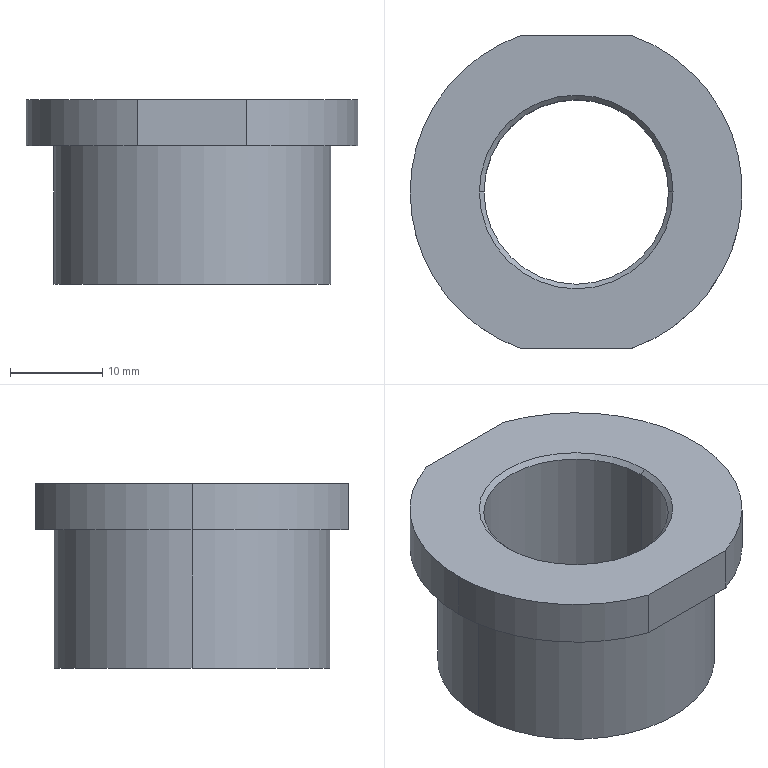Part | SolidWorks | features Chamfer 1, Extrusion 1, ICE 1 | 1 solid | 16 faces | box 36 x 34 x 20 mm | volume 9314 mm3 | cylinder 7 | plane 5 | cone 4 | commonest cylinder face diameters 36 x3 20 x2 30 x2
STEP:
#1=CARTESIAN_POINT('',(-10.,0.,19.5));
#2=VERTEX_POINT('',#1);
#3=CARTESIAN_POINT('',(10.,0.,19.5));
#4=VERTEX_POINT('',#3);
#5=CARTESIAN_POINT('',(0.,0.,19.5));
#6=DIRECTION('',(0.,0.,1.));
#7=DIRECTION('',(1.,0.,0.));
#8=AXIS2_PLACEMENT_3D('',#5,#6,#7);
#9=CIRCLE('',#8,10.);
#10=EDGE_CURVE('',#2,#4,#9,.T.);
#11=ORIENTED_EDGE('',*,*,#10,.F.);
#12=CARTESIAN_POINT('',(-10.5,0.,20.));
#13=VERTEX_POINT('',#12);
#14=CARTESIAN_POINT('',(-10.,0.,19.5));
#15=DIRECTION('',(-0.7071,0.,0.7071));
#16=VECTOR('',#15,1000.);
#17=LINE('',#14,#16);
#18=EDGE_CURVE('',#2,#13,#17,.T.);
#19=ORIENTED_EDGE('',*,*,#18,.T.);
#20=CARTESIAN_POINT('',(10.5,0.,20.));
#21=VERTEX_POINT('',#20);
#22=CARTESIAN_POINT('',(0.,0.,20.));
#23=DIRECTION('',(0.,0.,-1.));
#24=DIRECTION('',(1.,0.,0.));
#25=AXIS2_PLACEMENT_3D('',#22,#23,#24);
#26=CIRCLE('',#25,10.5);
#27=EDGE_CURVE('',#21,#13,#26,.T.);
#28=ORIENTED_EDGE('',*,*,#27,.F.);
#29=CARTESIAN_POINT('',(10.,0.,19.5));
#30=DIRECTION('',(0.7071,0.,0.7071));
#31=VECTOR('',#30,1000.);
#32=LINE('',#29,#31);
#33=EDGE_CURVE('',#4,#21,#32,.T.);
#34=ORIENTED_EDGE('',*,*,#33,.F.);
#35=EDGE_LOOP('',(#11,#19,#28,#34));
#36=FACE_OUTER_BOUND('',#35,.T.);
#37=CARTESIAN_POINT('',(0.,0.,19.5));
#38=DIRECTION('',(0.,0.,1.));
#39=DIRECTION('',(1.,0.,0.));
#40=AXIS2_PLACEMENT_3D('',#37,#38,#39);
#41=CONICAL_SURFACE('',#40,10.,0.7854);
#42=ADVANCED_FACE('',(#36),#41,.F.);
#43=CARTESIAN_POINT('',(10.,0.,0.5));
#44=VERTEX_POINT('',#43);
#45=CARTESIAN_POINT('',(-10.,0.,0.5));
#46=VERTEX_POINT('',#45);
#47=CARTESIAN_POINT('',(0.,0.,0.5));
#48=DIRECTION('',(0.,0.,-1.));
#49=DIRECTION('',(1.,0.,0.));
#50=AXIS2_PLACEMENT_3D('',#47,#48,#49);
#51=CIRCLE('',#50,10.);
#52=EDGE_CURVE('',#44,#46,#51,.T.);
#53=ORIENTED_EDGE('',*,*,#52,.F.);
#54=CARTESIAN_POINT('',(10.5,0.,0.));
#55=VERTEX_POINT('',#54);
#56=CARTESIAN_POINT('',(10.5,0.,0.));
#57=DIRECTION('',(0.7071,0.,-0.7071));
#58=VECTOR('',#57,1000.);
#59=LINE('',#56,#58);
#60=EDGE_CURVE('',#44,#55,#59,.T.);
#61=ORIENTED_EDGE('',*,*,#60,.T.);
#62=CARTESIAN_POINT('',(-10.5,0.,0.));
#63=VERTEX_POINT('',#62);
#64=CARTESIAN_POINT('',(0.,0.,0.));
#65=DIRECTION('',(0.,0.,1.));
#66=DIRECTION('',(1.,0.,0.));
#67=AXIS2_PLACEMENT_3D('',#64,#65,#66);
#68=CIRCLE('',#67,10.5);
#69=EDGE_CURVE('',#63,#55,#68,.T.);
#70=ORIENTED_EDGE('',*,*,#69,.F.);
#71=CARTESIAN_POINT('',(-10.5,0.,0.));
#72=DIRECTION('',(-0.7071,0.,-0.7071));
#73=VECTOR('',#72,1000.);
#74=LINE('',#71,#73);
#75=EDGE_CURVE('',#46,#63,#74,.T.);
#76=ORIENTED_EDGE('',*,*,#75,.F.);
#77=EDGE_LOOP('',(#53,#61,#70,#76));
#78=FACE_OUTER_BOUND('',#77,.T.);
#79=CARTESIAN_POINT('',(0.,0.,0.));
#80=DIRECTION('',(0.,0.,-1.));
#81=DIRECTION('',(-1.,0.,0.));
#82=AXIS2_PLACEMENT_3D('',#79,#80,#81);
#83=CONICAL_SURFACE('',#82,10.5,0.7854);
#84=ADVANCED_FACE('',(#78),#83,.F.);
#85=CARTESIAN_POINT('',(-18.,0.,20.));
#86=VERTEX_POINT('',#85);
#87=CARTESIAN_POINT('',(-5.916,-17.,20.));
#88=VERTEX_POINT('',#87);
#89=CARTESIAN_POINT('',(0.,0.,20.));
#90=DIRECTION('',(0.,0.,1.));
#91=DIRECTION('',(1.,0.,0.));
#92=AXIS2_PLACEMENT_3D('',#89,#90,#91);
#93=CIRCLE('',#92,18.);
#94=EDGE_CURVE('',#86,#88,#93,.T.);
#95=ORIENTED_EDGE('',*,*,#94,.F.);
#96=CARTESIAN_POINT('',(-18.,0.,15.));
#97=VERTEX_POINT('',#96);
#98=CARTESIAN_POINT('',(-18.,0.,20.));
#99=DIRECTION('',(0.,0.,-1.));
#100=VECTOR('',#99,1000.);
#101=LINE('',#98,#100);
#102=EDGE_CURVE('',#86,#97,#101,.T.);
#103=ORIENTED_EDGE('',*,*,#102,.T.);
#104=CARTESIAN_POINT('',(-5.916,-17.,15.));
#105=VERTEX_POINT('',#104);
#106=CARTESIAN_POINT('',(0.,0.,15.));
#107=DIRECTION('',(0.,0.,1.));
#108=DIRECTION('',(1.,0.,0.));
#109=AXIS2_PLACEMENT_3D('',#106,#107,#108);
#110=CIRCLE('',#109,18.);
#111=EDGE_CURVE('',#97,#105,#110,.T.);
#112=ORIENTED_EDGE('',*,*,#111,.T.);
#113=CARTESIAN_POINT('',(-5.916,-17.,20.));
#114=DIRECTION('',(0.,0.,-1.));
#115=VECTOR('',#114,1000.);
#116=LINE('',#113,#115);
#117=EDGE_CURVE('',#88,#105,#116,.T.);
#118=ORIENTED_EDGE('',*,*,#117,.F.);
#119=EDGE_LOOP('',(#95,#103,#112,#118));
#120=FACE_OUTER_BOUND('',#119,.T.);
#121=CARTESIAN_POINT('',(0.,0.,20.));
#122=DIRECTION('',(0.,0.,-1.));
#123=DIRECTION('',(-1.,0.,0.));
#124=AXIS2_PLACEMENT_3D('',#121,#122,#123);
#125=CYLINDRICAL_SURFACE('',#124,18.);
#126=ADVANCED_FACE('',(#120),#125,.T.);
#127=ORIENTED_EDGE('',*,*,#10,.T.);
#128=CARTESIAN_POINT('',(10.,0.,15.));
#129=DIRECTION('',(0.,0.,-1.));
#130=VECTOR('',#129,1000.);
#131=LINE('',#128,#130);
#132=EDGE_CURVE('',#4,#44,#131,.T.);
#133=ORIENTED_EDGE('',*,*,#132,.T.);
#134=ORIENTED_EDGE('',*,*,#52,.T.);
#135=CARTESIAN_POINT('',(-10.,0.,15.));
#136=DIRECTION('',(0.,0.,-1.));
#137=VECTOR('',#136,1000.);
#138=LINE('',#135,#137);
#139=EDGE_CURVE('',#2,#46,#138,.T.);
#140=ORIENTED_EDGE('',*,*,#139,.F.);
#141=EDGE_LOOP('',(#127,#133,#134,#140));
#142=FACE_OUTER_BOUND('',#141,.T.);
#143=CARTESIAN_POINT('',(0.,0.,15.));
#144=DIRECTION('',(0.,0.,-1.));
#145=DIRECTION('',(-1.,0.,0.));
#146=AXIS2_PLACEMENT_3D('',#143,#144,#145);
#147=CYLINDRICAL_SURFACE('',#146,10.);
#148=ADVANCED_FACE('',(#142),#147,.F.);
#149=CARTESIAN_POINT('',(15.,0.,15.));
#150=VERTEX_POINT('',#149);
#151=CARTESIAN_POINT('',(-15.,0.,15.));
#152=VERTEX_POINT('',#151);
#153=CARTESIAN_POINT('',(0.,0.,15.));
#154=DIRECTION('',(0.,0.,1.));
#155=DIRECTION('',(1.,0.,0.));
#156=AXIS2_PLACEMENT_3D('',#153,#154,#155);
#157=CIRCLE('',#156,15.);
#158=EDGE_CURVE('',#150,#152,#157,.T.);
#159=ORIENTED_EDGE('',*,*,#158,.F.);
#160=CARTESIAN_POINT('',(15.,0.,0.));
#161=VERTEX_POINT('',#160);
#162=CARTESIAN_POINT('',(15.,0.,15.));
#163=DIRECTION('',(0.,0.,-1.));
#164=VECTOR('',#163,1000.);
#165=LINE('',#162,#164);
#166=EDGE_CURVE('',#150,#161,#165,.T.);
#167=ORIENTED_EDGE('',*,*,#166,.T.);
#168=CARTESIAN_POINT('',(-15.,0.,0.));
#169=VERTEX_POINT('',#168);
#170=CARTESIAN_POINT('',(0.,0.,0.));
#171=DIRECTION('',(0.,0.,1.));
#172=DIRECTION('',(1.,0.,0.));
#173=AXIS2_PLACEMENT_3D('',#170,#171,#172);
#174=CIRCLE('',#173,15.);
#175=EDGE_CURVE('',#161,#169,#174,.T.);
#176=ORIENTED_EDGE('',*,*,#175,.T.);
#177=CARTESIAN_POINT('',(-15.,0.,15.));
#178=DIRECTION('',(0.,0.,-1.));
#179=VECTOR('',#178,1000.);
#180=LINE('',#177,#179);
#181=EDGE_CURVE('',#152,#169,#180,.T.);
#182=ORIENTED_EDGE('',*,*,#181,.F.);
#183=EDGE_LOOP('',(#159,#167,#176,#182));
#184=FACE_OUTER_BOUND('',#183,.T.);
#185=CARTESIAN_POINT('',(0.,0.,15.));
#186=DIRECTION('',(0.,0.,-1.));
#187=DIRECTION('',(-1.,0.,0.));
#188=AXIS2_PLACEMENT_3D('',#185,#186,#187);
#189=CYLINDRICAL_SURFACE('',#188,15.);
#190=ADVANCED_FACE('',(#184),#189,.T.);
#191=ORIENTED_EDGE('',*,*,#69,.T.);
#192=CARTESIAN_POINT('',(0.,0.,0.));
#193=DIRECTION('',(0.,0.,1.));
#194=DIRECTION('',(1.,0.,0.));
#195=AXIS2_PLACEMENT_3D('',#192,#193,#194);
#196=CIRCLE('',#195,10.5);
#197=EDGE_CURVE('',#55,#63,#196,.T.);
#198=ORIENTED_EDGE('',*,*,#197,.T.);
#199=EDGE_LOOP('',(#191,#198));
#200=FACE_BOUND('',#199,.T.);
#201=CARTESIAN_POINT('',(0.,0.,0.));
#202=DIRECTION('',(0.,0.,1.));
#203=DIRECTION('',(1.,0.,0.));
#204=AXIS2_PLACEMENT_3D('',#201,#202,#203);
#205=CIRCLE('',#204,15.);
#206=EDGE_CURVE('',#169,#161,#205,.T.);
#207=ORIENTED_EDGE('',*,*,#206,.F.);
#208=ORIENTED_EDGE('',*,*,#175,.F.);
#209=EDGE_LOOP('',(#207,#208));
#210=FACE_OUTER_BOUND('',#209,.T.);
#211=CARTESIAN_POINT('',(0.,0.,0.));
#212=DIRECTION('',(0.,0.,1.));
#213=DIRECTION('',(1.,0.,0.));
#214=AXIS2_PLACEMENT_3D('',#211,#212,#213);
#215=PLANE('',#214);
#216=ADVANCED_FACE('',(#200,#210),#215,.F.);
#217=ORIENTED_EDGE('',*,*,#166,.F.);
#218=CARTESIAN_POINT('',(0.,0.,15.));
#219=DIRECTION('',(0.,0.,1.));
#220=DIRECTION('',(1.,0.,0.));
#221=AXIS2_PLACEMENT_3D('',#218,#219,#220);
#222=CIRCLE('',#221,15.);
#223=EDGE_CURVE('',#152,#150,#222,.T.);
#224=ORIENTED_EDGE('',*,*,#223,.F.);
#225=ORIENTED_EDGE('',*,*,#181,.T.);
#226=ORIENTED_EDGE('',*,*,#206,.T.);
#227=EDGE_LOOP('',(#217,#224,#225,#226));
#228=FACE_OUTER_BOUND('',#227,.T.);
#229=CARTESIAN_POINT('',(0.,0.,15.));
#230=DIRECTION('',(0.,0.,-1.));
#231=DIRECTION('',(-1.,0.,0.));
#232=AXIS2_PLACEMENT_3D('',#229,#230,#231);
#233=CYLINDRICAL_SURFACE('',#232,15.);
#234=ADVANCED_FACE('',(#228),#233,.T.);
#235=ORIENTED_EDGE('',*,*,#132,.F.);
#236=CARTESIAN_POINT('',(0.,0.,19.5));
#237=DIRECTION('',(0.,0.,1.));
#238=DIRECTION('',(1.,0.,0.));
#239=AXIS2_PLACEMENT_3D('',#236,#237,#238);
#240=CIRCLE('',#239,10.);
#241=EDGE_CURVE('',#4,#2,#240,.T.);
#242=ORIENTED_EDGE('',*,*,#241,.T.);
#243=ORIENTED_EDGE('',*,*,#139,.T.);
#244=CARTESIAN_POINT('',(0.,0.,0.5));
#245=DIRECTION('',(0.,0.,-1.));
#246=DIRECTION('',(1.,0.,0.));
#247=AXIS2_PLACEMENT_3D('',#244,#245,#246);
#248=CIRCLE('',#247,10.);
#249=EDGE_CURVE('',#46,#44,#248,.T.);
#250=ORIENTED_EDGE('',*,*,#249,.T.);
#251=EDGE_LOOP('',(#235,#242,#243,#250));
#252=FACE_OUTER_BOUND('',#251,.T.);
#253=CARTESIAN_POINT('',(0.,0.,15.));
#254=DIRECTION('',(0.,0.,-1.));
#255=DIRECTION('',(-1.,0.,0.));
#256=AXIS2_PLACEMENT_3D('',#253,#254,#255);
#257=CYLINDRICAL_SURFACE('',#256,10.);
#258=ADVANCED_FACE('',(#252),#257,.F.);
#259=ORIENTED_EDGE('',*,*,#27,.T.);
#260=CARTESIAN_POINT('',(0.,0.,20.));
#261=DIRECTION('',(0.,0.,-1.));
#262=DIRECTION('',(1.,0.,0.));
#263=AXIS2_PLACEMENT_3D('',#260,#261,#262);
#264=CIRCLE('',#263,10.5);
#265=EDGE_CURVE('',#13,#21,#264,.T.);
#266=ORIENTED_EDGE('',*,*,#265,.T.);
#267=EDGE_LOOP('',(#259,#266));
#268=FACE_BOUND('',#267,.T.);
#269=CARTESIAN_POINT('',(-5.916,17.,20.));
#270=VERTEX_POINT('',#269);
#271=CARTESIAN_POINT('',(0.,0.,20.));
#272=DIRECTION('',(0.,0.,1.));
#273=DIRECTION('',(1.,0.,0.));
#274=AXIS2_PLACEMENT_3D('',#271,#272,#273);
#275=CIRCLE('',#274,18.);
#276=EDGE_CURVE('',#270,#86,#275,.T.);
#277=ORIENTED_EDGE('',*,*,#276,.T.);
#278=ORIENTED_EDGE('',*,*,#94,.T.);
#279=CARTESIAN_POINT('',(5.916,-17.,20.));
#280=VERTEX_POINT('',#279);
#281=CARTESIAN_POINT('',(-5.916,-17.,20.));
#282=DIRECTION('',(1.,0.,0.));
#283=VECTOR('',#282,1000.);
#284=LINE('',#281,#283);
#285=EDGE_CURVE('',#88,#280,#284,.T.);
#286=ORIENTED_EDGE('',*,*,#285,.T.);
#287=CARTESIAN_POINT('',(5.916,17.,20.));
#288=VERTEX_POINT('',#287);
#289=CARTESIAN_POINT('',(0.,0.,20.));
#290=DIRECTION('',(0.,0.,1.));
#291=DIRECTION('',(1.,0.,0.));
#292=AXIS2_PLACEMENT_3D('',#289,#290,#291);
#293=CIRCLE('',#292,18.);
#294=EDGE_CURVE('',#280,#288,#293,.T.);
#295=ORIENTED_EDGE('',*,*,#294,.T.);
#296=CARTESIAN_POINT('',(-5.916,17.,20.));
#297=DIRECTION('',(-1.,0.,0.));
#298=VECTOR('',#297,1000.);
#299=LINE('',#296,#298);
#300=EDGE_CURVE('',#288,#270,#299,.T.);
#301=ORIENTED_EDGE('',*,*,#300,.T.);
#302=EDGE_LOOP('',(#277,#278,#286,#295,#301));
#303=FACE_OUTER_BOUND('',#302,.T.);
#304=CARTESIAN_POINT('',(0.,0.,20.));
#305=DIRECTION('',(0.,0.,1.));
#306=DIRECTION('',(1.,0.,0.));
#307=AXIS2_PLACEMENT_3D('',#304,#305,#306);
#308=PLANE('',#307);
#309=ADVANCED_FACE('',(#268,#303),#308,.T.);
#310=ORIENTED_EDGE('',*,*,#223,.T.);
#311=ORIENTED_EDGE('',*,*,#158,.T.);
#312=EDGE_LOOP('',(#310,#311));
#313=FACE_BOUND('',#312,.T.);
#314=CARTESIAN_POINT('',(-5.916,17.,15.));
#315=VERTEX_POINT('',#314);
#316=CARTESIAN_POINT('',(0.,0.,15.));
#317=DIRECTION('',(0.,0.,1.));
#318=DIRECTION('',(1.,0.,0.));
#319=AXIS2_PLACEMENT_3D('',#316,#317,#318);
#320=CIRCLE('',#319,18.);
#321=EDGE_CURVE('',#315,#97,#320,.T.);
#322=ORIENTED_EDGE('',*,*,#321,.F.);
#323=CARTESIAN_POINT('',(5.916,17.,15.));
#324=VERTEX_POINT('',#323);
#325=CARTESIAN_POINT('',(-5.916,17.,15.));
#326=DIRECTION('',(-1.,0.,0.));
#327=VECTOR('',#326,1000.);
#328=LINE('',#325,#327);
#329=EDGE_CURVE('',#324,#315,#328,.T.);
#330=ORIENTED_EDGE('',*,*,#329,.F.);
#331=CARTESIAN_POINT('',(5.916,-17.,15.));
#332=VERTEX_POINT('',#331);
#333=CARTESIAN_POINT('',(0.,0.,15.));
#334=DIRECTION('',(0.,0.,1.));
#335=DIRECTION('',(1.,0.,0.));
#336=AXIS2_PLACEMENT_3D('',#333,#334,#335);
#337=CIRCLE('',#336,18.);
#338=EDGE_CURVE('',#332,#324,#337,.T.);
#339=ORIENTED_EDGE('',*,*,#338,.F.);
#340=CARTESIAN_POINT('',(-5.916,-17.,15.));
#341=DIRECTION('',(1.,0.,0.));
#342=VECTOR('',#341,1000.);
#343=LINE('',#340,#342);
#344=EDGE_CURVE('',#105,#332,#343,.T.);
#345=ORIENTED_EDGE('',*,*,#344,.F.);
#346=ORIENTED_EDGE('',*,*,#111,.F.);
#347=EDGE_LOOP('',(#322,#330,#339,#345,#346));
#348=FACE_OUTER_BOUND('',#347,.T.);
#349=CARTESIAN_POINT('',(0.,0.,15.));
#350=DIRECTION('',(0.,0.,1.));
#351=DIRECTION('',(1.,0.,0.));
#352=AXIS2_PLACEMENT_3D('',#349,#350,#351);
#353=PLANE('',#352);
#354=ADVANCED_FACE('',(#313,#348),#353,.F.);
#355=ORIENTED_EDGE('',*,*,#102,.F.);
#356=ORIENTED_EDGE('',*,*,#276,.F.);
#357=CARTESIAN_POINT('',(-5.916,17.,20.));
#358=DIRECTION('',(0.,0.,-1.));
#359=VECTOR('',#358,1000.);
#360=LINE('',#357,#359);
#361=EDGE_CURVE('',#270,#315,#360,.T.);
#362=ORIENTED_EDGE('',*,*,#361,.T.);
#363=ORIENTED_EDGE('',*,*,#321,.T.);
#364=EDGE_LOOP('',(#355,#356,#362,#363));
#365=FACE_OUTER_BOUND('',#364,.T.);
#366=CARTESIAN_POINT('',(0.,0.,20.));
#367=DIRECTION('',(0.,0.,-1.));
#368=DIRECTION('',(-1.,0.,0.));
#369=AXIS2_PLACEMENT_3D('',#366,#367,#368);
#370=CYLINDRICAL_SURFACE('',#369,18.);
#371=ADVANCED_FACE('',(#365),#370,.T.);
#372=ORIENTED_EDGE('',*,*,#344,.T.);
#373=CARTESIAN_POINT('',(5.916,-17.,20.));
#374=DIRECTION('',(0.,0.,-1.));
#375=VECTOR('',#374,1000.);
#376=LINE('',#373,#375);
#377=EDGE_CURVE('',#280,#332,#376,.T.);
#378=ORIENTED_EDGE('',*,*,#377,.F.);
#379=ORIENTED_EDGE('',*,*,#285,.F.);
#380=ORIENTED_EDGE('',*,*,#117,.T.);
#381=EDGE_LOOP('',(#372,#378,#379,#380));
#382=FACE_OUTER_BOUND('',#381,.T.);
#383=CARTESIAN_POINT('',(-5.916,-17.,20.));
#384=DIRECTION('',(0.,1.,0.));
#385=DIRECTION('',(0.,0.,1.));
#386=AXIS2_PLACEMENT_3D('',#383,#384,#385);
#387=PLANE('',#386);
#388=ADVANCED_FACE('',(#382),#387,.F.);
#389=ORIENTED_EDGE('',*,*,#338,.T.);
#390=CARTESIAN_POINT('',(5.916,17.,20.));
#391=DIRECTION('',(0.,0.,-1.));
#392=VECTOR('',#391,1000.);
#393=LINE('',#390,#392);
#394=EDGE_CURVE('',#288,#324,#393,.T.);
#395=ORIENTED_EDGE('',*,*,#394,.F.);
#396=ORIENTED_EDGE('',*,*,#294,.F.);
#397=ORIENTED_EDGE('',*,*,#377,.T.);
#398=EDGE_LOOP('',(#389,#395,#396,#397));
#399=FACE_OUTER_BOUND('',#398,.T.);
#400=CARTESIAN_POINT('',(0.,0.,20.));
#401=DIRECTION('',(0.,0.,-1.));
#402=DIRECTION('',(-1.,0.,0.));
#403=AXIS2_PLACEMENT_3D('',#400,#401,#402);
#404=CYLINDRICAL_SURFACE('',#403,18.);
#405=ADVANCED_FACE('',(#399),#404,.T.);
#406=ORIENTED_EDGE('',*,*,#329,.T.);
#407=ORIENTED_EDGE('',*,*,#361,.F.);
#408=ORIENTED_EDGE('',*,*,#300,.F.);
#409=ORIENTED_EDGE('',*,*,#394,.T.);
#410=EDGE_LOOP('',(#406,#407,#408,#409));
#411=FACE_OUTER_BOUND('',#410,.T.);
#412=CARTESIAN_POINT('',(-5.916,17.,20.));
#413=DIRECTION('',(0.,-1.,0.));
#414=DIRECTION('',(0.,0.,-1.));
#415=AXIS2_PLACEMENT_3D('',#412,#413,#414);
#416=PLANE('',#415);
#417=ADVANCED_FACE('',(#411),#416,.F.);
#418=ORIENTED_EDGE('',*,*,#60,.F.);
#419=ORIENTED_EDGE('',*,*,#249,.F.);
#420=ORIENTED_EDGE('',*,*,#75,.T.);
#421=ORIENTED_EDGE('',*,*,#197,.F.);
#422=EDGE_LOOP('',(#418,#419,#420,#421));
#423=FACE_OUTER_BOUND('',#422,.T.);
#424=CARTESIAN_POINT('',(0.,0.,0.));
#425=DIRECTION('',(0.,0.,-1.));
#426=DIRECTION('',(-1.,0.,0.));
#427=AXIS2_PLACEMENT_3D('',#424,#425,#426);
#428=CONICAL_SURFACE('',#427,10.5,0.7854);
#429=ADVANCED_FACE('',(#423),#428,.F.);
#430=ORIENTED_EDGE('',*,*,#18,.F.);
#431=ORIENTED_EDGE('',*,*,#241,.F.);
#432=ORIENTED_EDGE('',*,*,#33,.T.);
#433=ORIENTED_EDGE('',*,*,#265,.F.);
#434=EDGE_LOOP('',(#430,#431,#432,#433));
#435=FACE_OUTER_BOUND('',#434,.T.);
#436=CARTESIAN_POINT('',(0.,0.,19.5));
#437=DIRECTION('',(0.,0.,1.));
#438=DIRECTION('',(1.,0.,0.));
#439=AXIS2_PLACEMENT_3D('',#436,#437,#438);
#440=CONICAL_SURFACE('',#439,10.,0.7854);
#441=ADVANCED_FACE('',(#435),#440,.F.);
#442=CLOSED_SHELL('',(#42,#84,#126,#148,#190,#216,#234,#258,#309,#354,#371,#388,#405,#417,#429,#441));
#443=MANIFOLD_SOLID_BREP('',#442);
#444=CARTESIAN_POINT('',(0.,0.,0.));
#445=DIRECTION('',(0.,0.,1.));
#446=DIRECTION('',(1.,0.,0.));
#447=AXIS2_PLACEMENT_3D('',#444,#445,#446);
#448=(LENGTH_UNIT()NAMED_UNIT(*)SI_UNIT(.MILLI.,.METRE.));
#449=UNCERTAINTY_MEASURE_WITH_UNIT(LENGTH_MEASURE(0.00001),#448,'','');
#450=(NAMED_UNIT(*)PLANE_ANGLE_UNIT()SI_UNIT($,.RADIAN.));
#451=(NAMED_UNIT(*)SI_UNIT($,.STERADIAN.)SOLID_ANGLE_UNIT());
#452=(GEOMETRIC_REPRESENTATION_CONTEXT(3)GLOBAL_UNCERTAINTY_ASSIGNED_CONTEXT((#449))GLOBAL_UNIT_ASSIGNED_CONTEXT((#448,#450,#451))REPRESENTATION_CONTEXT('',''));
#453=ADVANCED_BREP_SHAPE_REPRESENTATION('',(#443,#447),#452);